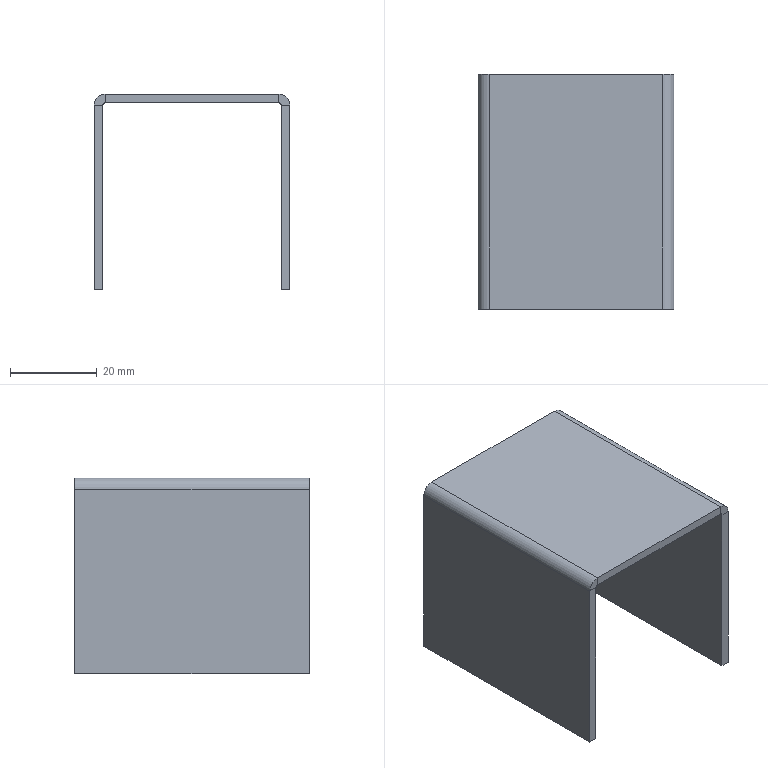Part | SolidWorks | features EdgeFlange 1, FlatPattern 1, SMBaseFlange 1, SheetMetal 1 | 1 solid | 22 faces | box 45 x 54 x 45 mm | volume 14009 mm3 | plane 18 | cylinder 4 | commonest cylinder face diameters 1 x2 5 x2
STEP:
#1=CARTESIAN_POINT('',(20.,-27.,-2.));
#2=VERTEX_POINT('',#1);
#3=CARTESIAN_POINT('',(20.,27.,-2.));
#4=VERTEX_POINT('',#3);
#5=CARTESIAN_POINT('',(20.,-27.,-2.));
#6=DIRECTION('',(0.,1.,0.));
#7=VECTOR('',#6,1000.);
#8=LINE('',#5,#7);
#9=EDGE_CURVE('',#2,#4,#8,.T.);
#10=ORIENTED_EDGE('',*,*,#9,.F.);
#11=CARTESIAN_POINT('',(-20.,-27.,-2.));
#12=VERTEX_POINT('',#11);
#13=CARTESIAN_POINT('',(-22.5,-27.,-2.));
#14=DIRECTION('',(1.,0.,0.));
#15=VECTOR('',#14,1000.);
#16=LINE('',#13,#15);
#17=EDGE_CURVE('',#12,#2,#16,.T.);
#18=ORIENTED_EDGE('',*,*,#17,.F.);
#19=CARTESIAN_POINT('',(-20.,27.,-2.));
#20=VERTEX_POINT('',#19);
#21=CARTESIAN_POINT('',(-20.,27.,-2.));
#22=DIRECTION('',(0.,-1.,0.));
#23=VECTOR('',#22,1000.);
#24=LINE('',#21,#23);
#25=EDGE_CURVE('',#20,#12,#24,.T.);
#26=ORIENTED_EDGE('',*,*,#25,.F.);
#27=CARTESIAN_POINT('',(-22.5,27.,-2.));
#28=DIRECTION('',(-1.,0.,0.));
#29=VECTOR('',#28,1000.);
#30=LINE('',#27,#29);
#31=EDGE_CURVE('',#4,#20,#30,.T.);
#32=ORIENTED_EDGE('',*,*,#31,.F.);
#33=EDGE_LOOP('',(#10,#18,#26,#32));
#34=FACE_OUTER_BOUND('',#33,.T.);
#35=CARTESIAN_POINT('',(0.,0.,-2.));
#36=DIRECTION('',(0.,0.,1.));
#37=DIRECTION('',(1.,0.,0.));
#38=AXIS2_PLACEMENT_3D('',#35,#36,#37);
#39=PLANE('',#38);
#40=ADVANCED_FACE('',(#34),#39,.F.);
#41=CARTESIAN_POINT('',(-20.,-27.,0.));
#42=VERTEX_POINT('',#41);
#43=CARTESIAN_POINT('',(20.,-27.,0.));
#44=VERTEX_POINT('',#43);
#45=CARTESIAN_POINT('',(-22.5,-27.,0.));
#46=DIRECTION('',(1.,0.,0.));
#47=VECTOR('',#46,1000.);
#48=LINE('',#45,#47);
#49=EDGE_CURVE('',#42,#44,#48,.T.);
#50=ORIENTED_EDGE('',*,*,#49,.T.);
#51=CARTESIAN_POINT('',(20.,27.,0.));
#52=VERTEX_POINT('',#51);
#53=CARTESIAN_POINT('',(20.,-27.,0.));
#54=DIRECTION('',(0.,1.,0.));
#55=VECTOR('',#54,1000.);
#56=LINE('',#53,#55);
#57=EDGE_CURVE('',#44,#52,#56,.T.);
#58=ORIENTED_EDGE('',*,*,#57,.T.);
#59=CARTESIAN_POINT('',(-20.,27.,0.));
#60=VERTEX_POINT('',#59);
#61=CARTESIAN_POINT('',(-22.5,27.,0.));
#62=DIRECTION('',(-1.,0.,0.));
#63=VECTOR('',#62,1000.);
#64=LINE('',#61,#63);
#65=EDGE_CURVE('',#52,#60,#64,.T.);
#66=ORIENTED_EDGE('',*,*,#65,.T.);
#67=CARTESIAN_POINT('',(-20.,27.,0.));
#68=DIRECTION('',(0.,-1.,0.));
#69=VECTOR('',#68,1000.);
#70=LINE('',#67,#69);
#71=EDGE_CURVE('',#60,#42,#70,.T.);
#72=ORIENTED_EDGE('',*,*,#71,.T.);
#73=EDGE_LOOP('',(#50,#58,#66,#72));
#74=FACE_OUTER_BOUND('',#73,.T.);
#75=CARTESIAN_POINT('',(0.,0.,0.));
#76=DIRECTION('',(0.,0.,1.));
#77=DIRECTION('',(1.,0.,0.));
#78=AXIS2_PLACEMENT_3D('',#75,#76,#77);
#79=PLANE('',#78);
#80=ADVANCED_FACE('',(#74),#79,.T.);
#81=ORIENTED_EDGE('',*,*,#17,.T.);
#82=CARTESIAN_POINT('',(20.,-27.,-2.));
#83=DIRECTION('',(0.,0.,1.));
#84=VECTOR('',#83,1000.);
#85=LINE('',#82,#84);
#86=EDGE_CURVE('',#2,#44,#85,.T.);
#87=ORIENTED_EDGE('',*,*,#86,.T.);
#88=ORIENTED_EDGE('',*,*,#49,.F.);
#89=CARTESIAN_POINT('',(-20.,-27.,-2.));
#90=DIRECTION('',(0.,0.,1.));
#91=VECTOR('',#90,1000.);
#92=LINE('',#89,#91);
#93=EDGE_CURVE('',#12,#42,#92,.T.);
#94=ORIENTED_EDGE('',*,*,#93,.F.);
#95=EDGE_LOOP('',(#81,#87,#88,#94));
#96=FACE_OUTER_BOUND('',#95,.T.);
#97=CARTESIAN_POINT('',(-22.5,-27.,-2.));
#98=DIRECTION('',(0.,-1.,0.));
#99=DIRECTION('',(0.,0.,-1.));
#100=AXIS2_PLACEMENT_3D('',#97,#98,#99);
#101=PLANE('',#100);
#102=ADVANCED_FACE('',(#96),#101,.T.);
#103=CARTESIAN_POINT('',(20.,27.,-2.));
#104=DIRECTION('',(0.,0.,1.));
#105=VECTOR('',#104,1000.);
#106=LINE('',#103,#105);
#107=EDGE_CURVE('',#4,#52,#106,.T.);
#108=ORIENTED_EDGE('',*,*,#107,.F.);
#109=ORIENTED_EDGE('',*,*,#31,.T.);
#110=CARTESIAN_POINT('',(-20.,27.,-2.));
#111=DIRECTION('',(0.,0.,1.));
#112=VECTOR('',#111,1000.);
#113=LINE('',#110,#112);
#114=EDGE_CURVE('',#20,#60,#113,.T.);
#115=ORIENTED_EDGE('',*,*,#114,.T.);
#116=ORIENTED_EDGE('',*,*,#65,.F.);
#117=EDGE_LOOP('',(#108,#109,#115,#116));
#118=FACE_OUTER_BOUND('',#117,.T.);
#119=CARTESIAN_POINT('',(-22.5,27.,-2.));
#120=DIRECTION('',(0.,1.,0.));
#121=DIRECTION('',(0.,0.,1.));
#122=AXIS2_PLACEMENT_3D('',#119,#120,#121);
#123=PLANE('',#122);
#124=ADVANCED_FACE('',(#118),#123,.T.);
#125=CARTESIAN_POINT('',(-20.5,-27.,-2.5));
#126=VERTEX_POINT('',#125);
#127=CARTESIAN_POINT('',(-22.5,-27.,-2.5));
#128=VERTEX_POINT('',#127);
#129=CARTESIAN_POINT('',(-22.5,-27.,-2.5));
#130=DIRECTION('',(-1.,0.,0.));
#131=VECTOR('',#130,1000.);
#132=LINE('',#129,#131);
#133=EDGE_CURVE('',#126,#128,#132,.T.);
#134=ORIENTED_EDGE('',*,*,#133,.F.);
#135=CARTESIAN_POINT('',(-20.,-27.,-2.5));
#136=DIRECTION('',(0.,-1.,0.));
#137=DIRECTION('',(0.,0.,1.));
#138=AXIS2_PLACEMENT_3D('',#135,#136,#137);
#139=CIRCLE('',#138,0.5);
#140=EDGE_CURVE('',#12,#126,#139,.T.);
#141=ORIENTED_EDGE('',*,*,#140,.F.);
#142=ORIENTED_EDGE('',*,*,#93,.T.);
#143=CARTESIAN_POINT('',(-20.,-27.,-2.5));
#144=DIRECTION('',(0.,-1.,0.));
#145=DIRECTION('',(0.,0.,1.));
#146=AXIS2_PLACEMENT_3D('',#143,#144,#145);
#147=CIRCLE('',#146,2.5);
#148=EDGE_CURVE('',#42,#128,#147,.T.);
#149=ORIENTED_EDGE('',*,*,#148,.T.);
#150=EDGE_LOOP('',(#134,#141,#142,#149));
#151=FACE_OUTER_BOUND('',#150,.T.);
#152=CARTESIAN_POINT('',(-20.,-27.,-2.5));
#153=DIRECTION('',(0.,-1.,0.));
#154=DIRECTION('',(0.,0.,-1.));
#155=AXIS2_PLACEMENT_3D('',#152,#153,#154);
#156=PLANE('',#155);
#157=ADVANCED_FACE('',(#151),#156,.T.);
#158=CARTESIAN_POINT('',(-20.5,27.,-2.5));
#159=VERTEX_POINT('',#158);
#160=CARTESIAN_POINT('',(-20.,27.,-2.5));
#161=DIRECTION('',(0.,1.,0.));
#162=DIRECTION('',(0.,0.,1.));
#163=AXIS2_PLACEMENT_3D('',#160,#161,#162);
#164=CIRCLE('',#163,0.5);
#165=EDGE_CURVE('',#159,#20,#164,.T.);
#166=ORIENTED_EDGE('',*,*,#165,.F.);
#167=CARTESIAN_POINT('',(-22.5,27.,-2.5));
#168=VERTEX_POINT('',#167);
#169=CARTESIAN_POINT('',(-20.5,27.,-2.5));
#170=DIRECTION('',(-1.,0.,0.));
#171=VECTOR('',#170,1000.);
#172=LINE('',#169,#171);
#173=EDGE_CURVE('',#159,#168,#172,.T.);
#174=ORIENTED_EDGE('',*,*,#173,.T.);
#175=CARTESIAN_POINT('',(-20.,27.,-2.5));
#176=DIRECTION('',(0.,1.,0.));
#177=DIRECTION('',(0.,0.,1.));
#178=AXIS2_PLACEMENT_3D('',#175,#176,#177);
#179=CIRCLE('',#178,2.5);
#180=EDGE_CURVE('',#168,#60,#179,.T.);
#181=ORIENTED_EDGE('',*,*,#180,.T.);
#182=ORIENTED_EDGE('',*,*,#114,.F.);
#183=EDGE_LOOP('',(#166,#174,#181,#182));
#184=FACE_OUTER_BOUND('',#183,.T.);
#185=CARTESIAN_POINT('',(-20.,27.,-2.5));
#186=DIRECTION('',(0.,-1.,0.));
#187=DIRECTION('',(0.,0.,-1.));
#188=AXIS2_PLACEMENT_3D('',#185,#186,#187);
#189=PLANE('',#188);
#190=ADVANCED_FACE('',(#184),#189,.F.);
#191=ORIENTED_EDGE('',*,*,#71,.F.);
#192=ORIENTED_EDGE('',*,*,#180,.F.);
#193=CARTESIAN_POINT('',(-22.5,0.,-2.5));
#194=DIRECTION('',(0.,1.,0.));
#195=VECTOR('',#194,1000.);
#196=LINE('',#193,#195);
#197=EDGE_CURVE('',#128,#168,#196,.T.);
#198=ORIENTED_EDGE('',*,*,#197,.F.);
#199=ORIENTED_EDGE('',*,*,#148,.F.);
#200=EDGE_LOOP('',(#191,#192,#198,#199));
#201=FACE_OUTER_BOUND('',#200,.T.);
#202=CARTESIAN_POINT('',(-20.,27.,-2.5));
#203=DIRECTION('',(0.,1.,0.));
#204=DIRECTION('',(-1.,0.,0.));
#205=AXIS2_PLACEMENT_3D('',#202,#203,#204);
#206=CYLINDRICAL_SURFACE('',#205,2.5);
#207=ADVANCED_FACE('',(#201),#206,.T.);
#208=ORIENTED_EDGE('',*,*,#25,.T.);
#209=ORIENTED_EDGE('',*,*,#140,.T.);
#210=CARTESIAN_POINT('',(-20.5,-27.,-2.5));
#211=DIRECTION('',(0.,1.,0.));
#212=VECTOR('',#211,1000.);
#213=LINE('',#210,#212);
#214=EDGE_CURVE('',#126,#159,#213,.T.);
#215=ORIENTED_EDGE('',*,*,#214,.T.);
#216=ORIENTED_EDGE('',*,*,#165,.T.);
#217=EDGE_LOOP('',(#208,#209,#215,#216));
#218=FACE_OUTER_BOUND('',#217,.T.);
#219=CARTESIAN_POINT('',(-20.,27.,-2.5));
#220=DIRECTION('',(0.,1.,0.));
#221=DIRECTION('',(-1.,0.,0.));
#222=AXIS2_PLACEMENT_3D('',#219,#220,#221);
#223=CYLINDRICAL_SURFACE('',#222,0.5);
#224=ADVANCED_FACE('',(#218),#223,.F.);
#225=CARTESIAN_POINT('',(-22.5,27.,-45.));
#226=VERTEX_POINT('',#225);
#227=CARTESIAN_POINT('',(-22.5,27.,-2.));
#228=DIRECTION('',(0.,0.,1.));
#229=VECTOR('',#228,1000.);
#230=LINE('',#227,#229);
#231=EDGE_CURVE('',#226,#168,#230,.T.);
#232=ORIENTED_EDGE('',*,*,#231,.T.);
#233=ORIENTED_EDGE('',*,*,#173,.F.);
#234=CARTESIAN_POINT('',(-20.5,27.,-45.));
#235=VERTEX_POINT('',#234);
#236=CARTESIAN_POINT('',(-20.5,27.,0.));
#237=DIRECTION('',(0.,0.,1.));
#238=VECTOR('',#237,1000.);
#239=LINE('',#236,#238);
#240=EDGE_CURVE('',#235,#159,#239,.T.);
#241=ORIENTED_EDGE('',*,*,#240,.F.);
#242=CARTESIAN_POINT('',(-22.5,27.,-45.));
#243=DIRECTION('',(1.,0.,0.));
#244=VECTOR('',#243,1000.);
#245=LINE('',#242,#244);
#246=EDGE_CURVE('',#226,#235,#245,.T.);
#247=ORIENTED_EDGE('',*,*,#246,.F.);
#248=EDGE_LOOP('',(#232,#233,#241,#247));
#249=FACE_OUTER_BOUND('',#248,.T.);
#250=CARTESIAN_POINT('',(-22.5,27.,-2.));
#251=DIRECTION('',(0.,1.,0.));
#252=DIRECTION('',(-1.,0.,0.));
#253=AXIS2_PLACEMENT_3D('',#250,#251,#252);
#254=PLANE('',#253);
#255=ADVANCED_FACE('',(#249),#254,.T.);
#256=CARTESIAN_POINT('',(-20.5,-27.,-45.));
#257=VERTEX_POINT('',#256);
#258=CARTESIAN_POINT('',(-20.5,-27.,0.));
#259=DIRECTION('',(0.,0.,-1.));
#260=VECTOR('',#259,1000.);
#261=LINE('',#258,#260);
#262=EDGE_CURVE('',#126,#257,#261,.T.);
#263=ORIENTED_EDGE('',*,*,#262,.F.);
#264=ORIENTED_EDGE('',*,*,#133,.T.);
#265=CARTESIAN_POINT('',(-22.5,-27.,-45.));
#266=VERTEX_POINT('',#265);
#267=CARTESIAN_POINT('',(-22.5,-27.,-45.));
#268=DIRECTION('',(0.,0.,-1.));
#269=VECTOR('',#268,1000.);
#270=LINE('',#267,#269);
#271=EDGE_CURVE('',#128,#266,#270,.T.);
#272=ORIENTED_EDGE('',*,*,#271,.T.);
#273=CARTESIAN_POINT('',(-22.5,-27.,-45.));
#274=DIRECTION('',(1.,0.,0.));
#275=VECTOR('',#274,1000.);
#276=LINE('',#273,#275);
#277=EDGE_CURVE('',#266,#257,#276,.T.);
#278=ORIENTED_EDGE('',*,*,#277,.T.);
#279=EDGE_LOOP('',(#263,#264,#272,#278));
#280=FACE_OUTER_BOUND('',#279,.T.);
#281=CARTESIAN_POINT('',(-22.5,-27.,-45.));
#282=DIRECTION('',(0.,-1.,0.));
#283=DIRECTION('',(1.,0.,0.));
#284=AXIS2_PLACEMENT_3D('',#281,#282,#283);
#285=PLANE('',#284);
#286=ADVANCED_FACE('',(#280),#285,.T.);
#287=ORIENTED_EDGE('',*,*,#271,.F.);
#288=ORIENTED_EDGE('',*,*,#197,.T.);
#289=ORIENTED_EDGE('',*,*,#231,.F.);
#290=CARTESIAN_POINT('',(-22.5,27.,-45.));
#291=DIRECTION('',(0.,1.,0.));
#292=VECTOR('',#291,1000.);
#293=LINE('',#290,#292);
#294=EDGE_CURVE('',#266,#226,#293,.T.);
#295=ORIENTED_EDGE('',*,*,#294,.F.);
#296=EDGE_LOOP('',(#287,#288,#289,#295));
#297=FACE_OUTER_BOUND('',#296,.T.);
#298=CARTESIAN_POINT('',(-22.5,0.,0.));
#299=DIRECTION('',(-1.,0.,0.));
#300=DIRECTION('',(0.,0.,1.));
#301=AXIS2_PLACEMENT_3D('',#298,#299,#300);
#302=PLANE('',#301);
#303=ADVANCED_FACE('',(#297),#302,.T.);
#304=ORIENTED_EDGE('',*,*,#214,.F.);
#305=ORIENTED_EDGE('',*,*,#262,.T.);
#306=CARTESIAN_POINT('',(-20.5,0.,-45.));
#307=DIRECTION('',(0.,1.,0.));
#308=VECTOR('',#307,1000.);
#309=LINE('',#306,#308);
#310=EDGE_CURVE('',#257,#235,#309,.T.);
#311=ORIENTED_EDGE('',*,*,#310,.T.);
#312=ORIENTED_EDGE('',*,*,#240,.T.);
#313=EDGE_LOOP('',(#304,#305,#311,#312));
#314=FACE_OUTER_BOUND('',#313,.T.);
#315=CARTESIAN_POINT('',(-20.5,0.,0.));
#316=DIRECTION('',(-1.,0.,0.));
#317=DIRECTION('',(0.,0.,1.));
#318=AXIS2_PLACEMENT_3D('',#315,#316,#317);
#319=PLANE('',#318);
#320=ADVANCED_FACE('',(#314),#319,.F.);
#321=ORIENTED_EDGE('',*,*,#310,.F.);
#322=ORIENTED_EDGE('',*,*,#277,.F.);
#323=ORIENTED_EDGE('',*,*,#294,.T.);
#324=ORIENTED_EDGE('',*,*,#246,.T.);
#325=EDGE_LOOP('',(#321,#322,#323,#324));
#326=FACE_OUTER_BOUND('',#325,.T.);
#327=CARTESIAN_POINT('',(-22.5,27.,-45.));
#328=DIRECTION('',(0.,0.,-1.));
#329=DIRECTION('',(-1.,0.,0.));
#330=AXIS2_PLACEMENT_3D('',#327,#328,#329);
#331=PLANE('',#330);
#332=ADVANCED_FACE('',(#326),#331,.T.);
#333=CARTESIAN_POINT('',(20.5,27.,-2.5));
#334=VERTEX_POINT('',#333);
#335=CARTESIAN_POINT('',(22.5,27.,-2.5));
#336=VERTEX_POINT('',#335);
#337=CARTESIAN_POINT('',(22.5,27.,-2.5));
#338=DIRECTION('',(1.,0.,0.));
#339=VECTOR('',#338,1000.);
#340=LINE('',#337,#339);
#341=EDGE_CURVE('',#334,#336,#340,.T.);
#342=ORIENTED_EDGE('',*,*,#341,.F.);
#343=CARTESIAN_POINT('',(20.,27.,-2.5));
#344=DIRECTION('',(0.,1.,0.));
#345=DIRECTION('',(0.,0.,-1.));
#346=AXIS2_PLACEMENT_3D('',#343,#344,#345);
#347=CIRCLE('',#346,0.5);
#348=EDGE_CURVE('',#4,#334,#347,.T.);
#349=ORIENTED_EDGE('',*,*,#348,.F.);
#350=ORIENTED_EDGE('',*,*,#107,.T.);
#351=CARTESIAN_POINT('',(20.,27.,-2.5));
#352=DIRECTION('',(0.,1.,0.));
#353=DIRECTION('',(0.,0.,-1.));
#354=AXIS2_PLACEMENT_3D('',#351,#352,#353);
#355=CIRCLE('',#354,2.5);
#356=EDGE_CURVE('',#52,#336,#355,.T.);
#357=ORIENTED_EDGE('',*,*,#356,.T.);
#358=EDGE_LOOP('',(#342,#349,#350,#357));
#359=FACE_OUTER_BOUND('',#358,.T.);
#360=CARTESIAN_POINT('',(20.,27.,-2.5));
#361=DIRECTION('',(0.,1.,0.));
#362=DIRECTION('',(0.,0.,1.));
#363=AXIS2_PLACEMENT_3D('',#360,#361,#362);
#364=PLANE('',#363);
#365=ADVANCED_FACE('',(#359),#364,.T.);
#366=CARTESIAN_POINT('',(20.5,-27.,-2.5));
#367=VERTEX_POINT('',#366);
#368=CARTESIAN_POINT('',(20.,-27.,-2.5));
#369=DIRECTION('',(0.,-1.,0.));
#370=DIRECTION('',(0.,0.,-1.));
#371=AXIS2_PLACEMENT_3D('',#368,#369,#370);
#372=CIRCLE('',#371,0.5);
#373=EDGE_CURVE('',#367,#2,#372,.T.);
#374=ORIENTED_EDGE('',*,*,#373,.F.);
#375=CARTESIAN_POINT('',(22.5,-27.,-2.5));
#376=VERTEX_POINT('',#375);
#377=CARTESIAN_POINT('',(20.5,-27.,-2.5));
#378=DIRECTION('',(1.,0.,0.));
#379=VECTOR('',#378,1000.);
#380=LINE('',#377,#379);
#381=EDGE_CURVE('',#367,#376,#380,.T.);
#382=ORIENTED_EDGE('',*,*,#381,.T.);
#383=CARTESIAN_POINT('',(20.,-27.,-2.5));
#384=DIRECTION('',(0.,-1.,0.));
#385=DIRECTION('',(0.,0.,-1.));
#386=AXIS2_PLACEMENT_3D('',#383,#384,#385);
#387=CIRCLE('',#386,2.5);
#388=EDGE_CURVE('',#376,#44,#387,.T.);
#389=ORIENTED_EDGE('',*,*,#388,.T.);
#390=ORIENTED_EDGE('',*,*,#86,.F.);
#391=EDGE_LOOP('',(#374,#382,#389,#390));
#392=FACE_OUTER_BOUND('',#391,.T.);
#393=CARTESIAN_POINT('',(20.,-27.,-2.5));
#394=DIRECTION('',(0.,1.,0.));
#395=DIRECTION('',(0.,0.,1.));
#396=AXIS2_PLACEMENT_3D('',#393,#394,#395);
#397=PLANE('',#396);
#398=ADVANCED_FACE('',(#392),#397,.F.);
#399=ORIENTED_EDGE('',*,*,#57,.F.);
#400=ORIENTED_EDGE('',*,*,#388,.F.);
#401=CARTESIAN_POINT('',(22.5,27.,-2.5));
#402=DIRECTION('',(0.,1.,0.));
#403=VECTOR('',#402,1000.);
#404=LINE('',#401,#403);
#405=EDGE_CURVE('',#376,#336,#404,.T.);
#406=ORIENTED_EDGE('',*,*,#405,.T.);
#407=ORIENTED_EDGE('',*,*,#356,.F.);
#408=EDGE_LOOP('',(#399,#400,#406,#407));
#409=FACE_OUTER_BOUND('',#408,.T.);
#410=CARTESIAN_POINT('',(20.,-27.,-2.5));
#411=DIRECTION('',(0.,-1.,0.));
#412=DIRECTION('',(1.,0.,0.));
#413=AXIS2_PLACEMENT_3D('',#410,#411,#412);
#414=CYLINDRICAL_SURFACE('',#413,2.5);
#415=ADVANCED_FACE('',(#409),#414,.T.);
#416=ORIENTED_EDGE('',*,*,#9,.T.);
#417=ORIENTED_EDGE('',*,*,#348,.T.);
#418=CARTESIAN_POINT('',(20.5,27.,-2.5));
#419=DIRECTION('',(0.,-1.,0.));
#420=VECTOR('',#419,1000.);
#421=LINE('',#418,#420);
#422=EDGE_CURVE('',#334,#367,#421,.T.);
#423=ORIENTED_EDGE('',*,*,#422,.T.);
#424=ORIENTED_EDGE('',*,*,#373,.T.);
#425=EDGE_LOOP('',(#416,#417,#423,#424));
#426=FACE_OUTER_BOUND('',#425,.T.);
#427=CARTESIAN_POINT('',(20.,-27.,-2.5));
#428=DIRECTION('',(0.,-1.,0.));
#429=DIRECTION('',(1.,0.,0.));
#430=AXIS2_PLACEMENT_3D('',#427,#428,#429);
#431=CYLINDRICAL_SURFACE('',#430,0.5);
#432=ADVANCED_FACE('',(#426),#431,.F.);
#433=CARTESIAN_POINT('',(20.5,27.,-45.));
#434=VERTEX_POINT('',#433);
#435=CARTESIAN_POINT('',(20.5,27.,0.));
#436=DIRECTION('',(0.,0.,-1.));
#437=VECTOR('',#436,1000.);
#438=LINE('',#435,#437);
#439=EDGE_CURVE('',#334,#434,#438,.T.);
#440=ORIENTED_EDGE('',*,*,#439,.F.);
#441=ORIENTED_EDGE('',*,*,#341,.T.);
#442=CARTESIAN_POINT('',(22.5,27.,-45.));
#443=VERTEX_POINT('',#442);
#444=CARTESIAN_POINT('',(22.5,27.,-2.));
#445=DIRECTION('',(0.,0.,-1.));
#446=VECTOR('',#445,1000.);
#447=LINE('',#444,#446);
#448=EDGE_CURVE('',#336,#443,#447,.T.);
#449=ORIENTED_EDGE('',*,*,#448,.T.);
#450=CARTESIAN_POINT('',(22.5,27.,-45.));
#451=DIRECTION('',(-1.,0.,0.));
#452=VECTOR('',#451,1000.);
#453=LINE('',#450,#452);
#454=EDGE_CURVE('',#443,#434,#453,.T.);
#455=ORIENTED_EDGE('',*,*,#454,.T.);
#456=EDGE_LOOP('',(#440,#441,#449,#455));
#457=FACE_OUTER_BOUND('',#456,.T.);
#458=CARTESIAN_POINT('',(22.5,27.,-2.));
#459=DIRECTION('',(0.,1.,0.));
#460=DIRECTION('',(-1.,0.,0.));
#461=AXIS2_PLACEMENT_3D('',#458,#459,#460);
#462=PLANE('',#461);
#463=ADVANCED_FACE('',(#457),#462,.T.);
#464=CARTESIAN_POINT('',(22.5,-27.,-45.));
#465=VERTEX_POINT('',#464);
#466=CARTESIAN_POINT('',(22.5,-27.,-45.));
#467=DIRECTION('',(0.,0.,1.));
#468=VECTOR('',#467,1000.);
#469=LINE('',#466,#468);
#470=EDGE_CURVE('',#465,#376,#469,.T.);
#471=ORIENTED_EDGE('',*,*,#470,.T.);
#472=ORIENTED_EDGE('',*,*,#381,.F.);
#473=CARTESIAN_POINT('',(20.5,-27.,-45.));
#474=VERTEX_POINT('',#473);
#475=CARTESIAN_POINT('',(20.5,-27.,0.));
#476=DIRECTION('',(0.,0.,1.));
#477=VECTOR('',#476,1000.);
#478=LINE('',#475,#477);
#479=EDGE_CURVE('',#474,#367,#478,.T.);
#480=ORIENTED_EDGE('',*,*,#479,.F.);
#481=CARTESIAN_POINT('',(22.5,-27.,-45.));
#482=DIRECTION('',(-1.,0.,0.));
#483=VECTOR('',#482,1000.);
#484=LINE('',#481,#483);
#485=EDGE_CURVE('',#465,#474,#484,.T.);
#486=ORIENTED_EDGE('',*,*,#485,.F.);
#487=EDGE_LOOP('',(#471,#472,#480,#486));
#488=FACE_OUTER_BOUND('',#487,.T.);
#489=CARTESIAN_POINT('',(22.5,-27.,-45.));
#490=DIRECTION('',(0.,-1.,0.));
#491=DIRECTION('',(1.,0.,0.));
#492=AXIS2_PLACEMENT_3D('',#489,#490,#491);
#493=PLANE('',#492);
#494=ADVANCED_FACE('',(#488),#493,.T.);
#495=ORIENTED_EDGE('',*,*,#405,.F.);
#496=ORIENTED_EDGE('',*,*,#470,.F.);
#497=CARTESIAN_POINT('',(22.5,27.,-45.));
#498=DIRECTION('',(0.,-1.,0.));
#499=VECTOR('',#498,1000.);
#500=LINE('',#497,#499);
#501=EDGE_CURVE('',#443,#465,#500,.T.);
#502=ORIENTED_EDGE('',*,*,#501,.F.);
#503=ORIENTED_EDGE('',*,*,#448,.F.);
#504=EDGE_LOOP('',(#495,#496,#502,#503));
#505=FACE_OUTER_BOUND('',#504,.T.);
#506=CARTESIAN_POINT('',(22.5,0.,0.));
#507=DIRECTION('',(-1.,0.,0.));
#508=DIRECTION('',(0.,0.,1.));
#509=AXIS2_PLACEMENT_3D('',#506,#507,#508);
#510=PLANE('',#509);
#511=ADVANCED_FACE('',(#505),#510,.F.);
#512=ORIENTED_EDGE('',*,*,#479,.T.);
#513=ORIENTED_EDGE('',*,*,#422,.F.);
#514=ORIENTED_EDGE('',*,*,#439,.T.);
#515=CARTESIAN_POINT('',(20.5,0.,-45.));
#516=DIRECTION('',(0.,-1.,0.));
#517=VECTOR('',#516,1000.);
#518=LINE('',#515,#517);
#519=EDGE_CURVE('',#434,#474,#518,.T.);
#520=ORIENTED_EDGE('',*,*,#519,.T.);
#521=EDGE_LOOP('',(#512,#513,#514,#520));
#522=FACE_OUTER_BOUND('',#521,.T.);
#523=CARTESIAN_POINT('',(20.5,0.,0.));
#524=DIRECTION('',(-1.,0.,0.));
#525=DIRECTION('',(0.,0.,1.));
#526=AXIS2_PLACEMENT_3D('',#523,#524,#525);
#527=PLANE('',#526);
#528=ADVANCED_FACE('',(#522),#527,.T.);
#529=ORIENTED_EDGE('',*,*,#519,.F.);
#530=ORIENTED_EDGE('',*,*,#454,.F.);
#531=ORIENTED_EDGE('',*,*,#501,.T.);
#532=ORIENTED_EDGE('',*,*,#485,.T.);
#533=EDGE_LOOP('',(#529,#530,#531,#532));
#534=FACE_OUTER_BOUND('',#533,.T.);
#535=CARTESIAN_POINT('',(22.5,27.,-45.));
#536=DIRECTION('',(0.,0.,-1.));
#537=DIRECTION('',(-1.,0.,0.));
#538=AXIS2_PLACEMENT_3D('',#535,#536,#537);
#539=PLANE('',#538);
#540=ADVANCED_FACE('',(#534),#539,.T.);
#541=CLOSED_SHELL('',(#40,#80,#102,#124,#157,#190,#207,#224,#255,#286,#303,#320,#332,#365,#398,#415,#432,#463,#494,#511,#528,#540));
#542=MANIFOLD_SOLID_BREP('',#541);
#543=CARTESIAN_POINT('',(0.,0.,0.));
#544=DIRECTION('',(0.,0.,1.));
#545=DIRECTION('',(1.,0.,0.));
#546=AXIS2_PLACEMENT_3D('',#543,#544,#545);
#547=(LENGTH_UNIT()NAMED_UNIT(*)SI_UNIT(.MILLI.,.METRE.));
#548=UNCERTAINTY_MEASURE_WITH_UNIT(LENGTH_MEASURE(0.00001),#547,'','');
#549=(NAMED_UNIT(*)PLANE_ANGLE_UNIT()SI_UNIT($,.RADIAN.));
#550=(NAMED_UNIT(*)SI_UNIT($,.STERADIAN.)SOLID_ANGLE_UNIT());
#551=(GEOMETRIC_REPRESENTATION_CONTEXT(3)GLOBAL_UNCERTAINTY_ASSIGNED_CONTEXT((#548))GLOBAL_UNIT_ASSIGNED_CONTEXT((#547,#549,#550))REPRESENTATION_CONTEXT('',''));
#552=ADVANCED_BREP_SHAPE_REPRESENTATION('',(#542,#546),#551);